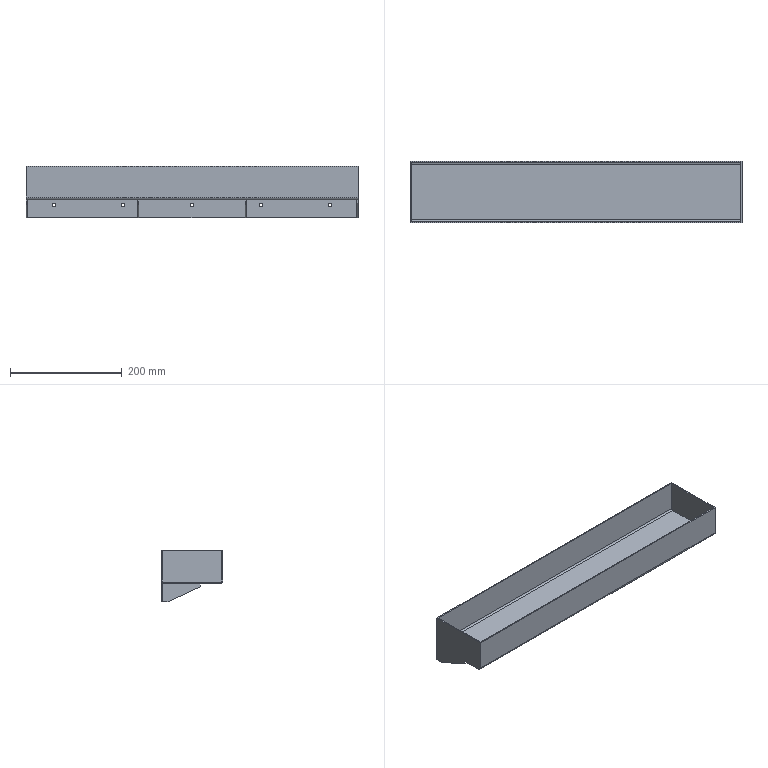Part | STEP file | Sheet metal material box | 1 solid | 45 faces | box 595 x 110 x 92 mm | volume 340939 mm3 | plane 29 | cylinder 16 | commonest cylinder face diameters 6.5 x10 10 x4 6 x2